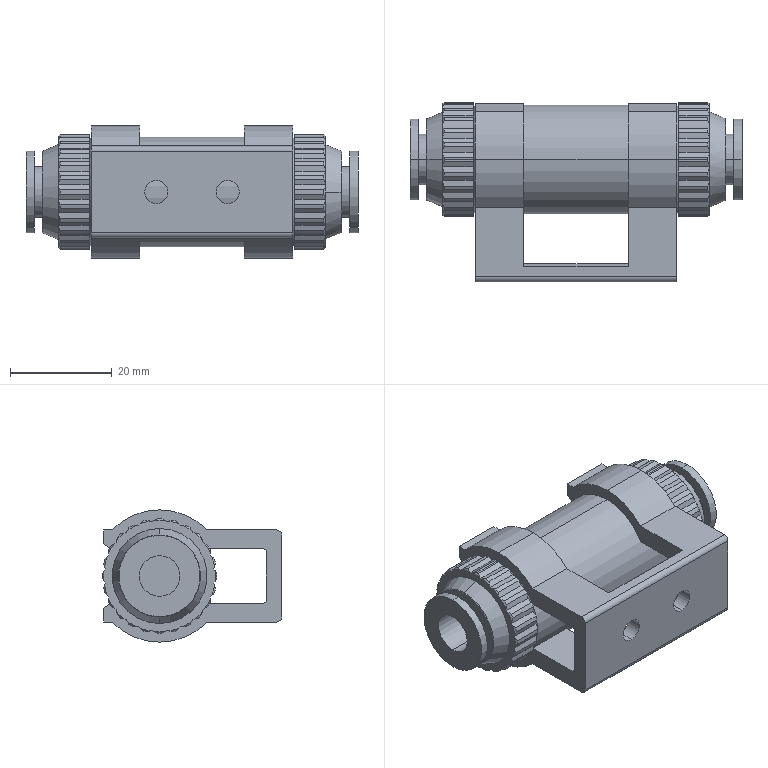Part | STEP file | VFD-03-08 | 1 solid | 278 faces | box 65.2 x 35.25 x 26 mm | volume 26161 mm3 | plane 138 | cylinder 78 | cone 58 | spline 4 | commonest cylinder face diameters 22.5 x50 26 x6 4.5 x4 8 x4 10 x4 16 x4